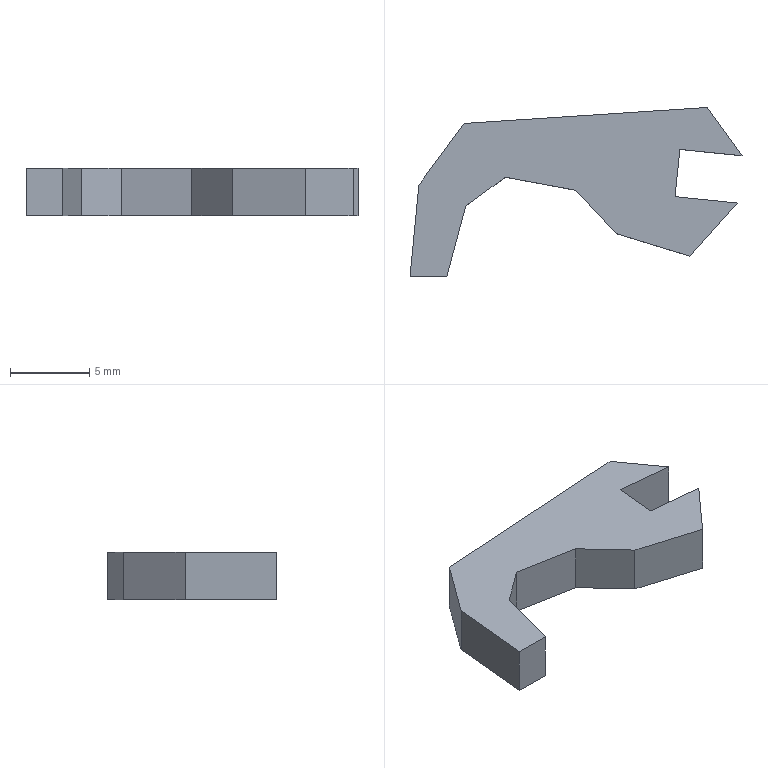Part | SolidWorks | features BaseBody 1 | 1 solid | 16 faces | box 20.938 x 10.659 x 3 mm | volume 345.483 mm3 | spline 9 | plane 7
STEP:
#1=CARTESIAN_POINT('',(78.769,3.624,-1.5));
#2=VERTEX_POINT('',#1);
#3=CARTESIAN_POINT('',(63.44,2.617,-1.5));
#4=VERTEX_POINT('',#3);
#5=CARTESIAN_POINT('',(78.769,3.624,-1.5));
#6=CARTESIAN_POINT('',(73.66,3.288,-1.5));
#7=CARTESIAN_POINT('',(68.549,2.953,-1.5));
#8=CARTESIAN_POINT('',(63.44,2.617,-1.5));
#9=B_SPLINE_CURVE_WITH_KNOTS('',3,(#5,#6,#7,#8),.UNSPECIFIED.,.F.,.F.,(4,4),(0.,0.04762),.UNSPECIFIED.);
#10=EDGE_CURVE('',#2,#4,#9,.T.);
#11=ORIENTED_EDGE('',*,*,#10,.F.);
#12=CARTESIAN_POINT('',(80.968,0.5797,-1.5));
#13=VERTEX_POINT('',#12);
#14=CARTESIAN_POINT('',(80.968,0.5797,-1.5));
#15=DIRECTION('',(-0.5856,0.8106,0.));
#16=VECTOR('',#15,1000.);
#17=LINE('',#14,#16);
#18=EDGE_CURVE('',#13,#2,#17,.T.);
#19=ORIENTED_EDGE('',*,*,#18,.F.);
#20=CARTESIAN_POINT('',(77.049,0.9807,-1.5));
#21=VERTEX_POINT('',#20);
#22=CARTESIAN_POINT('',(77.049,0.9807,-1.5));
#23=DIRECTION('',(0.9948,-0.1018,0.));
#24=VECTOR('',#23,1000.);
#25=LINE('',#22,#24);
#26=EDGE_CURVE('',#21,#13,#25,.T.);
#27=ORIENTED_EDGE('',*,*,#26,.F.);
#28=CARTESIAN_POINT('',(76.744,-2.004,-1.5));
#29=VERTEX_POINT('',#28);
#30=CARTESIAN_POINT('',(77.049,0.9807,-1.5));
#31=DIRECTION('',(0.1018,0.9948,0.));
#32=VECTOR('',#31,1000.);
#33=LINE('',#30,#32);
#34=EDGE_CURVE('',#29,#21,#33,.T.);
#35=ORIENTED_EDGE('',*,*,#34,.F.);
#36=CARTESIAN_POINT('',(80.656,-2.404,-1.5));
#37=VERTEX_POINT('',#36);
#38=CARTESIAN_POINT('',(76.744,-2.004,-1.5));
#39=DIRECTION('',(-0.9948,0.1018,0.));
#40=VECTOR('',#39,1000.);
#41=LINE('',#38,#40);
#42=EDGE_CURVE('',#37,#29,#41,.T.);
#43=ORIENTED_EDGE('',*,*,#42,.F.);
#44=CARTESIAN_POINT('',(77.656,-5.748,-1.5));
#45=VERTEX_POINT('',#44);
#46=CARTESIAN_POINT('',(77.656,-5.748,-1.5));
#47=CARTESIAN_POINT('',(78.655,-4.632,-1.5));
#48=CARTESIAN_POINT('',(80.656,-2.404,-1.5));
#49=B_SPLINE_CURVE_WITH_KNOTS('',2,(#46,#47,#48),.UNSPECIFIED.,.F.,.F.,(3,3),(0.4286,0.4762),.UNSPECIFIED.);
#50=EDGE_CURVE('',#45,#37,#49,.T.);
#51=ORIENTED_EDGE('',*,*,#50,.F.);
#52=CARTESIAN_POINT('',(73.035,-4.338,-1.5));
#53=VERTEX_POINT('',#52);
#54=CARTESIAN_POINT('',(73.035,-4.338,-1.5));
#55=DIRECTION('',(0.9564,-0.292,0.));
#56=VECTOR('',#55,1000.);
#57=LINE('',#54,#56);
#58=EDGE_CURVE('',#53,#45,#57,.T.);
#59=ORIENTED_EDGE('',*,*,#58,.F.);
#60=CARTESIAN_POINT('',(70.495,-1.597,-1.5));
#61=VERTEX_POINT('',#60);
#62=CARTESIAN_POINT('',(70.495,-1.597,-1.5));
#63=CARTESIAN_POINT('',(71.34,-2.51,-1.5));
#64=CARTESIAN_POINT('',(72.189,-3.425,-1.5));
#65=CARTESIAN_POINT('',(73.035,-4.338,-1.5));
#66=B_SPLINE_CURVE_WITH_KNOTS('',3,(#62,#63,#64,#65),.UNSPECIFIED.,.F.,.F.,(4,4),(0.3333,0.381),.UNSPECIFIED.);
#67=EDGE_CURVE('',#61,#53,#66,.T.);
#68=ORIENTED_EDGE('',*,*,#67,.F.);
#69=CARTESIAN_POINT('',(66.033,-0.7769,-1.5));
#70=VERTEX_POINT('',#69);
#71=CARTESIAN_POINT('',(66.033,-0.7769,-1.5));
#72=CARTESIAN_POINT('',(67.52,-1.049,-1.5));
#73=CARTESIAN_POINT('',(69.006,-1.323,-1.5));
#74=CARTESIAN_POINT('',(70.495,-1.597,-1.5));
#75=B_SPLINE_CURVE_WITH_KNOTS('',3,(#71,#72,#73,#74),.UNSPECIFIED.,.F.,.F.,(4,4),(0.2857,0.3333),.UNSPECIFIED.);
#76=EDGE_CURVE('',#70,#61,#75,.T.);
#77=ORIENTED_EDGE('',*,*,#76,.F.);
#78=CARTESIAN_POINT('',(63.538,-2.605,-1.5));
#79=VERTEX_POINT('',#78);
#80=CARTESIAN_POINT('',(63.538,-2.605,-1.5));
#81=CARTESIAN_POINT('',(64.37,-1.995,-1.5));
#82=CARTESIAN_POINT('',(65.202,-1.387,-1.5));
#83=CARTESIAN_POINT('',(66.033,-0.7769,-1.5));
#84=B_SPLINE_CURVE_WITH_KNOTS('',3,(#80,#81,#82,#83),.UNSPECIFIED.,.F.,.F.,(4,4),(0.2381,0.2857),.UNSPECIFIED.);
#85=EDGE_CURVE('',#79,#70,#84,.T.);
#86=ORIENTED_EDGE('',*,*,#85,.F.);
#87=CARTESIAN_POINT('',(62.352,-7.033,-1.5));
#88=VERTEX_POINT('',#87);
#89=CARTESIAN_POINT('',(62.352,-7.033,-1.5));
#90=CARTESIAN_POINT('',(62.747,-5.557,-1.5));
#91=CARTESIAN_POINT('',(63.143,-4.081,-1.5));
#92=CARTESIAN_POINT('',(63.538,-2.605,-1.5));
#93=B_SPLINE_CURVE_WITH_KNOTS('',3,(#89,#90,#91,#92),.UNSPECIFIED.,.F.,.F.,(4,4),(0.1905,0.2381),.UNSPECIFIED.);
#94=EDGE_CURVE('',#88,#79,#93,.T.);
#95=ORIENTED_EDGE('',*,*,#94,.F.);
#96=CARTESIAN_POINT('',(60.03,-7.035,-1.5));
#97=VERTEX_POINT('',#96);
#98=CARTESIAN_POINT('',(60.03,-7.035,-1.5));
#99=CARTESIAN_POINT('',(60.803,-7.033,-1.5));
#100=CARTESIAN_POINT('',(61.577,-7.033,-1.5));
#101=CARTESIAN_POINT('',(62.352,-7.033,-1.5));
#102=B_SPLINE_CURVE_WITH_KNOTS('',3,(#98,#99,#100,#101),.UNSPECIFIED.,.F.,.F.,(4,4),(0.1429,0.1905),.UNSPECIFIED.);
#103=EDGE_CURVE('',#97,#88,#102,.T.);
#104=ORIENTED_EDGE('',*,*,#103,.F.);
#105=CARTESIAN_POINT('',(60.588,-1.271,-1.5));
#106=VERTEX_POINT('',#105);
#107=CARTESIAN_POINT('',(60.588,-1.271,-1.5));
#108=CARTESIAN_POINT('',(60.401,-3.192,-1.5));
#109=CARTESIAN_POINT('',(60.217,-5.114,-1.5));
#110=CARTESIAN_POINT('',(60.03,-7.035,-1.5));
#111=B_SPLINE_CURVE_WITH_KNOTS('',3,(#107,#108,#109,#110),.UNSPECIFIED.,.F.,.F.,(4,4),(0.09524,0.1429),.UNSPECIFIED.);
#112=EDGE_CURVE('',#106,#97,#111,.T.);
#113=ORIENTED_EDGE('',*,*,#112,.F.);
#114=CARTESIAN_POINT('',(63.44,2.617,-1.5));
#115=CARTESIAN_POINT('',(62.49,1.321,-1.5));
#116=CARTESIAN_POINT('',(61.539,0.02496,-1.5));
#117=CARTESIAN_POINT('',(60.588,-1.271,-1.5));
#118=B_SPLINE_CURVE_WITH_KNOTS('',3,(#114,#115,#116,#117),.UNSPECIFIED.,.F.,.F.,(4,4),(0.04762,0.09524),.UNSPECIFIED.);
#119=EDGE_CURVE('',#4,#106,#118,.T.);
#120=ORIENTED_EDGE('',*,*,#119,.F.);
#121=EDGE_LOOP('',(#11,#19,#27,#35,#43,#51,#59,#68,#77,#86,#95,#104,#113,#120));
#122=FACE_OUTER_BOUND('',#121,.T.);
#123=CARTESIAN_POINT('',(71.105,3.12,-1.5));
#124=DIRECTION('',(0.,0.,1.));
#125=DIRECTION('',(1.,0.,0.));
#126=AXIS2_PLACEMENT_3D('',#123,#124,#125);
#127=PLANE('',#126);
#128=ADVANCED_FACE('',(#122),#127,.F.);
#129=CARTESIAN_POINT('',(78.769,3.624,1.5));
#130=VERTEX_POINT('',#129);
#131=CARTESIAN_POINT('',(63.44,2.617,1.5));
#132=VERTEX_POINT('',#131);
#133=CARTESIAN_POINT('',(78.769,3.624,1.5));
#134=CARTESIAN_POINT('',(73.66,3.288,1.5));
#135=CARTESIAN_POINT('',(68.549,2.953,1.5));
#136=CARTESIAN_POINT('',(63.44,2.617,1.5));
#137=B_SPLINE_CURVE_WITH_KNOTS('',3,(#133,#134,#135,#136),.UNSPECIFIED.,.F.,.F.,(4,4),(0.,0.04762),.UNSPECIFIED.);
#138=EDGE_CURVE('',#130,#132,#137,.T.);
#139=ORIENTED_EDGE('',*,*,#138,.T.);
#140=CARTESIAN_POINT('',(60.588,-1.271,1.5));
#141=VERTEX_POINT('',#140);
#142=CARTESIAN_POINT('',(63.44,2.617,1.5));
#143=CARTESIAN_POINT('',(62.49,1.321,1.5));
#144=CARTESIAN_POINT('',(61.539,0.02496,1.5));
#145=CARTESIAN_POINT('',(60.588,-1.271,1.5));
#146=B_SPLINE_CURVE_WITH_KNOTS('',3,(#142,#143,#144,#145),.UNSPECIFIED.,.F.,.F.,(4,4),(0.04762,0.09524),.UNSPECIFIED.);
#147=EDGE_CURVE('',#132,#141,#146,.T.);
#148=ORIENTED_EDGE('',*,*,#147,.T.);
#149=CARTESIAN_POINT('',(60.03,-7.035,1.5));
#150=VERTEX_POINT('',#149);
#151=CARTESIAN_POINT('',(60.588,-1.271,1.5));
#152=CARTESIAN_POINT('',(60.401,-3.192,1.5));
#153=CARTESIAN_POINT('',(60.217,-5.114,1.5));
#154=CARTESIAN_POINT('',(60.03,-7.035,1.5));
#155=B_SPLINE_CURVE_WITH_KNOTS('',3,(#151,#152,#153,#154),.UNSPECIFIED.,.F.,.F.,(4,4),(0.09524,0.1429),.UNSPECIFIED.);
#156=EDGE_CURVE('',#141,#150,#155,.T.);
#157=ORIENTED_EDGE('',*,*,#156,.T.);
#158=CARTESIAN_POINT('',(62.352,-7.033,1.5));
#159=VERTEX_POINT('',#158);
#160=CARTESIAN_POINT('',(60.03,-7.035,1.5));
#161=CARTESIAN_POINT('',(60.803,-7.033,1.5));
#162=CARTESIAN_POINT('',(61.577,-7.033,1.5));
#163=CARTESIAN_POINT('',(62.352,-7.033,1.5));
#164=B_SPLINE_CURVE_WITH_KNOTS('',3,(#160,#161,#162,#163),.UNSPECIFIED.,.F.,.F.,(4,4),(0.1429,0.1905),.UNSPECIFIED.);
#165=EDGE_CURVE('',#150,#159,#164,.T.);
#166=ORIENTED_EDGE('',*,*,#165,.T.);
#167=CARTESIAN_POINT('',(63.538,-2.605,1.5));
#168=VERTEX_POINT('',#167);
#169=CARTESIAN_POINT('',(62.352,-7.033,1.5));
#170=CARTESIAN_POINT('',(62.747,-5.557,1.5));
#171=CARTESIAN_POINT('',(63.143,-4.081,1.5));
#172=CARTESIAN_POINT('',(63.538,-2.605,1.5));
#173=B_SPLINE_CURVE_WITH_KNOTS('',3,(#169,#170,#171,#172),.UNSPECIFIED.,.F.,.F.,(4,4),(0.1905,0.2381),.UNSPECIFIED.);
#174=EDGE_CURVE('',#159,#168,#173,.T.);
#175=ORIENTED_EDGE('',*,*,#174,.T.);
#176=CARTESIAN_POINT('',(66.033,-0.7769,1.5));
#177=VERTEX_POINT('',#176);
#178=CARTESIAN_POINT('',(63.538,-2.605,1.5));
#179=CARTESIAN_POINT('',(64.37,-1.995,1.5));
#180=CARTESIAN_POINT('',(65.202,-1.387,1.5));
#181=CARTESIAN_POINT('',(66.033,-0.7769,1.5));
#182=B_SPLINE_CURVE_WITH_KNOTS('',3,(#178,#179,#180,#181),.UNSPECIFIED.,.F.,.F.,(4,4),(0.2381,0.2857),.UNSPECIFIED.);
#183=EDGE_CURVE('',#168,#177,#182,.T.);
#184=ORIENTED_EDGE('',*,*,#183,.T.);
#185=CARTESIAN_POINT('',(70.495,-1.597,1.5));
#186=VERTEX_POINT('',#185);
#187=CARTESIAN_POINT('',(66.033,-0.7769,1.5));
#188=CARTESIAN_POINT('',(67.52,-1.049,1.5));
#189=CARTESIAN_POINT('',(69.006,-1.323,1.5));
#190=CARTESIAN_POINT('',(70.495,-1.597,1.5));
#191=B_SPLINE_CURVE_WITH_KNOTS('',3,(#187,#188,#189,#190),.UNSPECIFIED.,.F.,.F.,(4,4),(0.2857,0.3333),.UNSPECIFIED.);
#192=EDGE_CURVE('',#177,#186,#191,.T.);
#193=ORIENTED_EDGE('',*,*,#192,.T.);
#194=CARTESIAN_POINT('',(73.035,-4.338,1.5));
#195=VERTEX_POINT('',#194);
#196=CARTESIAN_POINT('',(70.495,-1.597,1.5));
#197=CARTESIAN_POINT('',(71.34,-2.51,1.5));
#198=CARTESIAN_POINT('',(72.189,-3.425,1.5));
#199=CARTESIAN_POINT('',(73.035,-4.338,1.5));
#200=B_SPLINE_CURVE_WITH_KNOTS('',3,(#196,#197,#198,#199),.UNSPECIFIED.,.F.,.F.,(4,4),(0.3333,0.381),.UNSPECIFIED.);
#201=EDGE_CURVE('',#186,#195,#200,.T.);
#202=ORIENTED_EDGE('',*,*,#201,.T.);
#203=CARTESIAN_POINT('',(77.656,-5.748,1.5));
#204=VERTEX_POINT('',#203);
#205=CARTESIAN_POINT('',(73.035,-4.338,1.5));
#206=DIRECTION('',(0.9564,-0.292,0.));
#207=VECTOR('',#206,1000.);
#208=LINE('',#205,#207);
#209=EDGE_CURVE('',#195,#204,#208,.T.);
#210=ORIENTED_EDGE('',*,*,#209,.T.);
#211=CARTESIAN_POINT('',(80.656,-2.404,1.5));
#212=VERTEX_POINT('',#211);
#213=CARTESIAN_POINT('',(77.656,-5.748,1.5));
#214=CARTESIAN_POINT('',(78.655,-4.632,1.5));
#215=CARTESIAN_POINT('',(80.656,-2.404,1.5));
#216=B_SPLINE_CURVE_WITH_KNOTS('',2,(#213,#214,#215),.UNSPECIFIED.,.F.,.F.,(3,3),(0.4286,0.4762),.UNSPECIFIED.);
#217=EDGE_CURVE('',#204,#212,#216,.T.);
#218=ORIENTED_EDGE('',*,*,#217,.T.);
#219=CARTESIAN_POINT('',(76.744,-2.004,1.5));
#220=VERTEX_POINT('',#219);
#221=CARTESIAN_POINT('',(76.744,-2.004,1.5));
#222=DIRECTION('',(-0.9948,0.1018,0.));
#223=VECTOR('',#222,1000.);
#224=LINE('',#221,#223);
#225=EDGE_CURVE('',#212,#220,#224,.T.);
#226=ORIENTED_EDGE('',*,*,#225,.T.);
#227=CARTESIAN_POINT('',(77.049,0.9807,1.5));
#228=VERTEX_POINT('',#227);
#229=CARTESIAN_POINT('',(77.049,0.9807,1.5));
#230=DIRECTION('',(0.1018,0.9948,0.));
#231=VECTOR('',#230,1000.);
#232=LINE('',#229,#231);
#233=EDGE_CURVE('',#220,#228,#232,.T.);
#234=ORIENTED_EDGE('',*,*,#233,.T.);
#235=CARTESIAN_POINT('',(80.968,0.5797,1.5));
#236=VERTEX_POINT('',#235);
#237=CARTESIAN_POINT('',(77.049,0.9807,1.5));
#238=DIRECTION('',(0.9948,-0.1018,0.));
#239=VECTOR('',#238,1000.);
#240=LINE('',#237,#239);
#241=EDGE_CURVE('',#228,#236,#240,.T.);
#242=ORIENTED_EDGE('',*,*,#241,.T.);
#243=CARTESIAN_POINT('',(80.968,0.5797,1.5));
#244=DIRECTION('',(-0.5856,0.8106,0.));
#245=VECTOR('',#244,1000.);
#246=LINE('',#243,#245);
#247=EDGE_CURVE('',#236,#130,#246,.T.);
#248=ORIENTED_EDGE('',*,*,#247,.T.);
#249=EDGE_LOOP('',(#139,#148,#157,#166,#175,#184,#193,#202,#210,#218,#226,#234,#242,#248));
#250=FACE_OUTER_BOUND('',#249,.T.);
#251=CARTESIAN_POINT('',(71.105,3.12,1.5));
#252=DIRECTION('',(0.,0.,1.));
#253=DIRECTION('',(1.,0.,0.));
#254=AXIS2_PLACEMENT_3D('',#251,#252,#253);
#255=PLANE('',#254);
#256=ADVANCED_FACE('',(#250),#255,.T.);
#257=ORIENTED_EDGE('',*,*,#18,.T.);
#258=CARTESIAN_POINT('',(78.769,3.624,1.5));
#259=DIRECTION('',(0.,0.,-1.));
#260=VECTOR('',#259,1000.);
#261=LINE('',#258,#260);
#262=EDGE_CURVE('',#130,#2,#261,.T.);
#263=ORIENTED_EDGE('',*,*,#262,.F.);
#264=ORIENTED_EDGE('',*,*,#247,.F.);
#265=CARTESIAN_POINT('',(80.968,0.5797,1.5));
#266=DIRECTION('',(0.,0.,-1.));
#267=VECTOR('',#266,1000.);
#268=LINE('',#265,#267);
#269=EDGE_CURVE('',#236,#13,#268,.T.);
#270=ORIENTED_EDGE('',*,*,#269,.T.);
#271=EDGE_LOOP('',(#257,#263,#264,#270));
#272=FACE_OUTER_BOUND('',#271,.T.);
#273=CARTESIAN_POINT('',(80.968,0.5797,1.5));
#274=DIRECTION('',(-0.8106,-0.5856,0.));
#275=DIRECTION('',(-0.5856,0.8106,0.));
#276=AXIS2_PLACEMENT_3D('',#273,#274,#275);
#277=PLANE('',#276);
#278=ADVANCED_FACE('',(#272),#277,.F.);
#279=ORIENTED_EDGE('',*,*,#26,.T.);
#280=ORIENTED_EDGE('',*,*,#269,.F.);
#281=ORIENTED_EDGE('',*,*,#241,.F.);
#282=CARTESIAN_POINT('',(77.049,0.9807,1.5));
#283=DIRECTION('',(0.,0.,-1.));
#284=VECTOR('',#283,1000.);
#285=LINE('',#282,#284);
#286=EDGE_CURVE('',#228,#21,#285,.T.);
#287=ORIENTED_EDGE('',*,*,#286,.T.);
#288=EDGE_LOOP('',(#279,#280,#281,#287));
#289=FACE_OUTER_BOUND('',#288,.T.);
#290=CARTESIAN_POINT('',(77.049,0.9807,1.5));
#291=DIRECTION('',(0.1018,0.9948,0.));
#292=DIRECTION('',(0.,0.,-1.));
#293=AXIS2_PLACEMENT_3D('',#290,#291,#292);
#294=PLANE('',#293);
#295=ADVANCED_FACE('',(#289),#294,.F.);
#296=ORIENTED_EDGE('',*,*,#34,.T.);
#297=ORIENTED_EDGE('',*,*,#286,.F.);
#298=ORIENTED_EDGE('',*,*,#233,.F.);
#299=CARTESIAN_POINT('',(76.744,-2.004,1.5));
#300=DIRECTION('',(0.,0.,-1.));
#301=VECTOR('',#300,1000.);
#302=LINE('',#299,#301);
#303=EDGE_CURVE('',#220,#29,#302,.T.);
#304=ORIENTED_EDGE('',*,*,#303,.T.);
#305=EDGE_LOOP('',(#296,#297,#298,#304));
#306=FACE_OUTER_BOUND('',#305,.T.);
#307=CARTESIAN_POINT('',(77.049,0.9807,1.5));
#308=DIRECTION('',(-0.9948,0.1018,0.));
#309=DIRECTION('',(0.,0.,1.));
#310=AXIS2_PLACEMENT_3D('',#307,#308,#309);
#311=PLANE('',#310);
#312=ADVANCED_FACE('',(#306),#311,.F.);
#313=ORIENTED_EDGE('',*,*,#42,.T.);
#314=ORIENTED_EDGE('',*,*,#303,.F.);
#315=ORIENTED_EDGE('',*,*,#225,.F.);
#316=CARTESIAN_POINT('',(80.656,-2.404,1.5));
#317=DIRECTION('',(0.,0.,-1.));
#318=VECTOR('',#317,1000.);
#319=LINE('',#316,#318);
#320=EDGE_CURVE('',#212,#37,#319,.T.);
#321=ORIENTED_EDGE('',*,*,#320,.T.);
#322=EDGE_LOOP('',(#313,#314,#315,#321));
#323=FACE_OUTER_BOUND('',#322,.T.);
#324=CARTESIAN_POINT('',(76.744,-2.004,1.5));
#325=DIRECTION('',(-0.1018,-0.9948,0.));
#326=DIRECTION('',(-0.9948,0.1018,0.));
#327=AXIS2_PLACEMENT_3D('',#324,#325,#326);
#328=PLANE('',#327);
#329=ADVANCED_FACE('',(#323),#328,.F.);
#330=ORIENTED_EDGE('',*,*,#50,.T.);
#331=ORIENTED_EDGE('',*,*,#320,.F.);
#332=ORIENTED_EDGE('',*,*,#217,.F.);
#333=CARTESIAN_POINT('',(77.656,-5.748,1.5));
#334=DIRECTION('',(0.,0.,-1.));
#335=VECTOR('',#334,1000.);
#336=LINE('',#333,#335);
#337=EDGE_CURVE('',#204,#45,#336,.T.);
#338=ORIENTED_EDGE('',*,*,#337,.T.);
#339=EDGE_LOOP('',(#330,#331,#332,#338));
#340=FACE_OUTER_BOUND('',#339,.T.);
#341=CARTESIAN_POINT('',(77.656,-5.748,1.5));
#342=CARTESIAN_POINT('',(77.656,-5.748,-1.5));
#343=CARTESIAN_POINT('',(78.655,-4.632,1.5));
#344=CARTESIAN_POINT('',(78.655,-4.632,-1.5));
#345=CARTESIAN_POINT('',(80.656,-2.404,1.5));
#346=CARTESIAN_POINT('',(80.656,-2.404,-1.5));
#347=B_SPLINE_SURFACE_WITH_KNOTS('',2,1,((#341,#342),(#343,#344),(#345,#346)),.UNSPECIFIED.,.F.,.F.,.F.,(3,3),(2,2),(0.4286,0.4762),(0.,1.),.UNSPECIFIED.);
#348=ADVANCED_FACE('',(#340),#347,.F.);
#349=ORIENTED_EDGE('',*,*,#58,.T.);
#350=ORIENTED_EDGE('',*,*,#337,.F.);
#351=ORIENTED_EDGE('',*,*,#209,.F.);
#352=CARTESIAN_POINT('',(73.035,-4.338,1.5));
#353=DIRECTION('',(0.,0.,-1.));
#354=VECTOR('',#353,1000.);
#355=LINE('',#352,#354);
#356=EDGE_CURVE('',#195,#53,#355,.T.);
#357=ORIENTED_EDGE('',*,*,#356,.T.);
#358=EDGE_LOOP('',(#349,#350,#351,#357));
#359=FACE_OUTER_BOUND('',#358,.T.);
#360=CARTESIAN_POINT('',(73.035,-4.338,1.5));
#361=DIRECTION('',(0.292,0.9564,0.));
#362=DIRECTION('',(0.,0.,-1.));
#363=AXIS2_PLACEMENT_3D('',#360,#361,#362);
#364=PLANE('',#363);
#365=ADVANCED_FACE('',(#359),#364,.F.);
#366=ORIENTED_EDGE('',*,*,#67,.T.);
#367=ORIENTED_EDGE('',*,*,#356,.F.);
#368=ORIENTED_EDGE('',*,*,#201,.F.);
#369=CARTESIAN_POINT('',(70.495,-1.597,1.5));
#370=DIRECTION('',(0.,0.,-1.));
#371=VECTOR('',#370,1000.);
#372=LINE('',#369,#371);
#373=EDGE_CURVE('',#186,#61,#372,.T.);
#374=ORIENTED_EDGE('',*,*,#373,.T.);
#375=EDGE_LOOP('',(#366,#367,#368,#374));
#376=FACE_OUTER_BOUND('',#375,.T.);
#377=CARTESIAN_POINT('',(70.495,-1.597,1.5));
#378=CARTESIAN_POINT('',(70.495,-1.597,-1.5));
#379=CARTESIAN_POINT('',(71.34,-2.51,1.5));
#380=CARTESIAN_POINT('',(71.34,-2.51,-1.5));
#381=CARTESIAN_POINT('',(72.189,-3.425,1.5));
#382=CARTESIAN_POINT('',(72.189,-3.425,-1.5));
#383=CARTESIAN_POINT('',(73.035,-4.338,1.5));
#384=CARTESIAN_POINT('',(73.035,-4.338,-1.5));
#385=B_SPLINE_SURFACE_WITH_KNOTS('',3,1,((#377,#378),(#379,#380),(#381,#382),(#383,#384)),.UNSPECIFIED.,.F.,.F.,.F.,(4,4),(2,2),(0.3333,0.381),(0.,1.),.UNSPECIFIED.);
#386=ADVANCED_FACE('',(#376),#385,.F.);
#387=ORIENTED_EDGE('',*,*,#76,.T.);
#388=ORIENTED_EDGE('',*,*,#373,.F.);
#389=ORIENTED_EDGE('',*,*,#192,.F.);
#390=CARTESIAN_POINT('',(66.033,-0.7769,1.5));
#391=DIRECTION('',(0.,0.,-1.));
#392=VECTOR('',#391,1000.);
#393=LINE('',#390,#392);
#394=EDGE_CURVE('',#177,#70,#393,.T.);
#395=ORIENTED_EDGE('',*,*,#394,.T.);
#396=EDGE_LOOP('',(#387,#388,#389,#395));
#397=FACE_OUTER_BOUND('',#396,.T.);
#398=CARTESIAN_POINT('',(66.033,-0.7769,1.5));
#399=CARTESIAN_POINT('',(66.033,-0.7769,-1.5));
#400=CARTESIAN_POINT('',(67.52,-1.049,1.5));
#401=CARTESIAN_POINT('',(67.52,-1.049,-1.5));
#402=CARTESIAN_POINT('',(69.006,-1.323,1.5));
#403=CARTESIAN_POINT('',(69.006,-1.323,-1.5));
#404=CARTESIAN_POINT('',(70.495,-1.597,1.5));
#405=CARTESIAN_POINT('',(70.495,-1.597,-1.5));
#406=B_SPLINE_SURFACE_WITH_KNOTS('',3,1,((#398,#399),(#400,#401),(#402,#403),(#404,#405)),.UNSPECIFIED.,.F.,.F.,.F.,(4,4),(2,2),(0.2857,0.3333),(0.,1.),.UNSPECIFIED.);
#407=ADVANCED_FACE('',(#397),#406,.F.);
#408=ORIENTED_EDGE('',*,*,#85,.T.);
#409=ORIENTED_EDGE('',*,*,#394,.F.);
#410=ORIENTED_EDGE('',*,*,#183,.F.);
#411=CARTESIAN_POINT('',(63.538,-2.605,1.5));
#412=DIRECTION('',(0.,0.,-1.));
#413=VECTOR('',#412,1000.);
#414=LINE('',#411,#413);
#415=EDGE_CURVE('',#168,#79,#414,.T.);
#416=ORIENTED_EDGE('',*,*,#415,.T.);
#417=EDGE_LOOP('',(#408,#409,#410,#416));
#418=FACE_OUTER_BOUND('',#417,.T.);
#419=CARTESIAN_POINT('',(63.538,-2.605,1.5));
#420=CARTESIAN_POINT('',(63.538,-2.605,-1.5));
#421=CARTESIAN_POINT('',(64.37,-1.995,1.5));
#422=CARTESIAN_POINT('',(64.37,-1.995,-1.5));
#423=CARTESIAN_POINT('',(65.202,-1.387,1.5));
#424=CARTESIAN_POINT('',(65.202,-1.387,-1.5));
#425=CARTESIAN_POINT('',(66.033,-0.7769,1.5));
#426=CARTESIAN_POINT('',(66.033,-0.7769,-1.5));
#427=B_SPLINE_SURFACE_WITH_KNOTS('',3,1,((#419,#420),(#421,#422),(#423,#424),(#425,#426)),.UNSPECIFIED.,.F.,.F.,.F.,(4,4),(2,2),(0.2381,0.2857),(0.,1.),.UNSPECIFIED.);
#428=ADVANCED_FACE('',(#418),#427,.F.);
#429=ORIENTED_EDGE('',*,*,#94,.T.);
#430=ORIENTED_EDGE('',*,*,#415,.F.);
#431=ORIENTED_EDGE('',*,*,#174,.F.);
#432=CARTESIAN_POINT('',(62.352,-7.033,1.5));
#433=DIRECTION('',(0.,0.,-1.));
#434=VECTOR('',#433,1000.);
#435=LINE('',#432,#434);
#436=EDGE_CURVE('',#159,#88,#435,.T.);
#437=ORIENTED_EDGE('',*,*,#436,.T.);
#438=EDGE_LOOP('',(#429,#430,#431,#437));
#439=FACE_OUTER_BOUND('',#438,.T.);
#440=CARTESIAN_POINT('',(62.352,-7.033,1.5));
#441=CARTESIAN_POINT('',(62.352,-7.033,-1.5));
#442=CARTESIAN_POINT('',(62.747,-5.557,1.5));
#443=CARTESIAN_POINT('',(62.747,-5.557,-1.5));
#444=CARTESIAN_POINT('',(63.143,-4.081,1.5));
#445=CARTESIAN_POINT('',(63.143,-4.081,-1.5));
#446=CARTESIAN_POINT('',(63.538,-2.605,1.5));
#447=CARTESIAN_POINT('',(63.538,-2.605,-1.5));
#448=B_SPLINE_SURFACE_WITH_KNOTS('',3,1,((#440,#441),(#442,#443),(#444,#445),(#446,#447)),.UNSPECIFIED.,.F.,.F.,.F.,(4,4),(2,2),(0.1905,0.2381),(0.,1.),.UNSPECIFIED.);
#449=ADVANCED_FACE('',(#439),#448,.F.);
#450=ORIENTED_EDGE('',*,*,#103,.T.);
#451=ORIENTED_EDGE('',*,*,#436,.F.);
#452=ORIENTED_EDGE('',*,*,#165,.F.);
#453=CARTESIAN_POINT('',(60.03,-7.035,1.5));
#454=DIRECTION('',(0.,0.,-1.));
#455=VECTOR('',#454,1000.);
#456=LINE('',#453,#455);
#457=EDGE_CURVE('',#150,#97,#456,.T.);
#458=ORIENTED_EDGE('',*,*,#457,.T.);
#459=EDGE_LOOP('',(#450,#451,#452,#458));
#460=FACE_OUTER_BOUND('',#459,.T.);
#461=CARTESIAN_POINT('',(60.03,-7.035,1.5));
#462=CARTESIAN_POINT('',(60.03,-7.035,-1.5));
#463=CARTESIAN_POINT('',(60.803,-7.033,1.5));
#464=CARTESIAN_POINT('',(60.803,-7.033,-1.5));
#465=CARTESIAN_POINT('',(61.577,-7.033,1.5));
#466=CARTESIAN_POINT('',(61.577,-7.033,-1.5));
#467=CARTESIAN_POINT('',(62.352,-7.033,1.5));
#468=CARTESIAN_POINT('',(62.352,-7.033,-1.5));
#469=B_SPLINE_SURFACE_WITH_KNOTS('',3,1,((#461,#462),(#463,#464),(#465,#466),(#467,#468)),.UNSPECIFIED.,.F.,.F.,.F.,(4,4),(2,2),(0.1429,0.1905),(0.,1.),.UNSPECIFIED.);
#470=ADVANCED_FACE('',(#460),#469,.F.);
#471=ORIENTED_EDGE('',*,*,#112,.T.);
#472=ORIENTED_EDGE('',*,*,#457,.F.);
#473=ORIENTED_EDGE('',*,*,#156,.F.);
#474=CARTESIAN_POINT('',(60.588,-1.271,1.5));
#475=DIRECTION('',(0.,0.,-1.));
#476=VECTOR('',#475,1000.);
#477=LINE('',#474,#476);
#478=EDGE_CURVE('',#141,#106,#477,.T.);
#479=ORIENTED_EDGE('',*,*,#478,.T.);
#480=EDGE_LOOP('',(#471,#472,#473,#479));
#481=FACE_OUTER_BOUND('',#480,.T.);
#482=CARTESIAN_POINT('',(60.588,-1.271,1.5));
#483=CARTESIAN_POINT('',(60.588,-1.271,-1.5));
#484=CARTESIAN_POINT('',(60.401,-3.192,1.5));
#485=CARTESIAN_POINT('',(60.401,-3.192,-1.5));
#486=CARTESIAN_POINT('',(60.217,-5.114,1.5));
#487=CARTESIAN_POINT('',(60.217,-5.114,-1.5));
#488=CARTESIAN_POINT('',(60.03,-7.035,1.5));
#489=CARTESIAN_POINT('',(60.03,-7.035,-1.5));
#490=B_SPLINE_SURFACE_WITH_KNOTS('',3,1,((#482,#483),(#484,#485),(#486,#487),(#488,#489)),.UNSPECIFIED.,.F.,.F.,.F.,(4,4),(2,2),(0.09524,0.1429),(0.,1.),.UNSPECIFIED.);
#491=ADVANCED_FACE('',(#481),#490,.F.);
#492=ORIENTED_EDGE('',*,*,#119,.T.);
#493=ORIENTED_EDGE('',*,*,#478,.F.);
#494=ORIENTED_EDGE('',*,*,#147,.F.);
#495=CARTESIAN_POINT('',(63.44,2.617,1.5));
#496=DIRECTION('',(0.,0.,-1.));
#497=VECTOR('',#496,1000.);
#498=LINE('',#495,#497);
#499=EDGE_CURVE('',#132,#4,#498,.T.);
#500=ORIENTED_EDGE('',*,*,#499,.T.);
#501=EDGE_LOOP('',(#492,#493,#494,#500));
#502=FACE_OUTER_BOUND('',#501,.T.);
#503=CARTESIAN_POINT('',(63.44,2.617,1.5));
#504=CARTESIAN_POINT('',(63.44,2.617,-1.5));
#505=CARTESIAN_POINT('',(62.49,1.321,1.5));
#506=CARTESIAN_POINT('',(62.49,1.321,-1.5));
#507=CARTESIAN_POINT('',(61.539,0.02496,1.5));
#508=CARTESIAN_POINT('',(61.539,0.02496,-1.5));
#509=CARTESIAN_POINT('',(60.588,-1.271,1.5));
#510=CARTESIAN_POINT('',(60.588,-1.271,-1.5));
#511=B_SPLINE_SURFACE_WITH_KNOTS('',3,1,((#503,#504),(#505,#506),(#507,#508),(#509,#510)),.UNSPECIFIED.,.F.,.F.,.F.,(4,4),(2,2),(0.04762,0.09524),(0.,1.),.UNSPECIFIED.);
#512=ADVANCED_FACE('',(#502),#511,.F.);
#513=ORIENTED_EDGE('',*,*,#10,.T.);
#514=ORIENTED_EDGE('',*,*,#499,.F.);
#515=ORIENTED_EDGE('',*,*,#138,.F.);
#516=ORIENTED_EDGE('',*,*,#262,.T.);
#517=EDGE_LOOP('',(#513,#514,#515,#516));
#518=FACE_OUTER_BOUND('',#517,.T.);
#519=CARTESIAN_POINT('',(78.769,3.624,1.5));
#520=CARTESIAN_POINT('',(78.769,3.624,-1.5));
#521=CARTESIAN_POINT('',(73.66,3.288,1.5));
#522=CARTESIAN_POINT('',(73.66,3.288,-1.5));
#523=CARTESIAN_POINT('',(68.549,2.953,1.5));
#524=CARTESIAN_POINT('',(68.549,2.953,-1.5));
#525=CARTESIAN_POINT('',(63.44,2.617,1.5));
#526=CARTESIAN_POINT('',(63.44,2.617,-1.5));
#527=B_SPLINE_SURFACE_WITH_KNOTS('',3,1,((#519,#520),(#521,#522),(#523,#524),(#525,#526)),.UNSPECIFIED.,.F.,.F.,.F.,(4,4),(2,2),(0.,0.04762),(0.,1.),.UNSPECIFIED.);
#528=ADVANCED_FACE('',(#518),#527,.F.);
#529=CLOSED_SHELL('',(#128,#256,#278,#295,#312,#329,#348,#365,#386,#407,#428,#449,#470,#491,#512,#528));
#530=MANIFOLD_SOLID_BREP('',#529);
#531=CARTESIAN_POINT('',(0.,0.,0.));
#532=DIRECTION('',(0.,0.,1.));
#533=DIRECTION('',(1.,0.,0.));
#534=AXIS2_PLACEMENT_3D('',#531,#532,#533);
#535=(LENGTH_UNIT()NAMED_UNIT(*)SI_UNIT(.MILLI.,.METRE.));
#536=UNCERTAINTY_MEASURE_WITH_UNIT(LENGTH_MEASURE(0.00001),#535,'','');
#537=(NAMED_UNIT(*)PLANE_ANGLE_UNIT()SI_UNIT($,.RADIAN.));
#538=(NAMED_UNIT(*)SI_UNIT($,.STERADIAN.)SOLID_ANGLE_UNIT());
#539=(GEOMETRIC_REPRESENTATION_CONTEXT(3)GLOBAL_UNCERTAINTY_ASSIGNED_CONTEXT((#536))GLOBAL_UNIT_ASSIGNED_CONTEXT((#535,#537,#538))REPRESENTATION_CONTEXT('',''));
#540=ADVANCED_BREP_SHAPE_REPRESENTATION('',(#530,#534),#539);